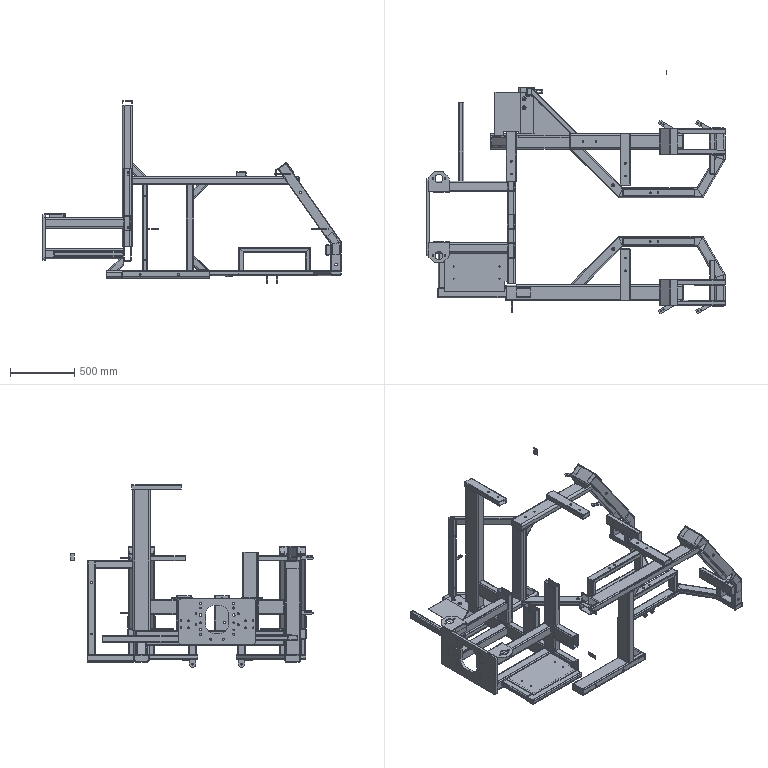Part | STEP file | COMPOUND | 108 solids | 1565 faces | box 2329 x 1902 x 1425 mm | volume 39311271 mm3 | plane 919 | cylinder 646 | commonest cylinder face diameters 20 x149 10 x148 12 x96 6 x91 14 x48 16 x16